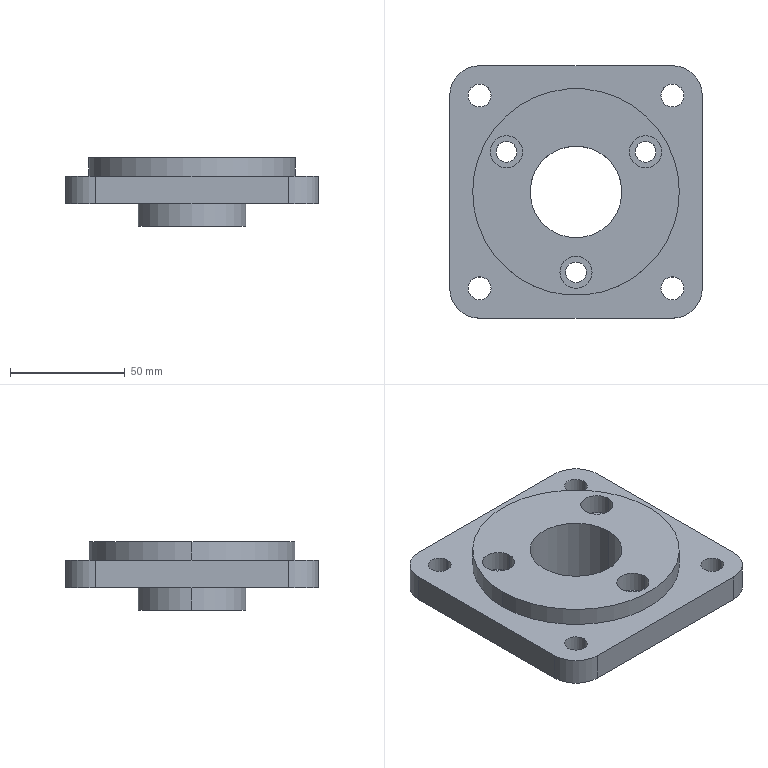Part | SolidWorks | features ICE 6, CirPattern 1, Extrusion 1 | 1 solid | 41 faces | box 110 x 110 x 29.8 mm | volume 163882 mm3 | cylinder 30 | plane 11 | commonest cylinder face diameters 10 x8 9 x6 14 x6 26 x4 40 x2 47 x2
STEP:
#1=CARTESIAN_POINT('',(-34.811,17.5,0.));
#2=VERTEX_POINT('',#1);
#3=CARTESIAN_POINT('',(-25.811,17.5,0.));
#4=VERTEX_POINT('',#3);
#5=CARTESIAN_POINT('',(-30.311,17.5,0.));
#6=DIRECTION('',(0.,0.,1.));
#7=DIRECTION('',(1.,0.,0.));
#8=AXIS2_PLACEMENT_3D('',#5,#6,#7);
#9=CIRCLE('',#8,4.5);
#10=EDGE_CURVE('',#2,#4,#9,.T.);
#11=ORIENTED_EDGE('',*,*,#10,.F.);
#12=CARTESIAN_POINT('',(-34.811,17.5,11.));
#13=VERTEX_POINT('',#12);
#14=CARTESIAN_POINT('',(-34.811,17.5,-790.));
#15=DIRECTION('',(0.,0.,1.));
#16=VECTOR('',#15,1000.);
#17=LINE('',#14,#16);
#18=EDGE_CURVE('',#2,#13,#17,.T.);
#19=ORIENTED_EDGE('',*,*,#18,.T.);
#20=CARTESIAN_POINT('',(-25.811,17.5,11.));
#21=VERTEX_POINT('',#20);
#22=CARTESIAN_POINT('',(-30.311,17.5,11.));
#23=DIRECTION('',(0.,0.,1.));
#24=DIRECTION('',(-0.5,-0.866,0.));
#25=AXIS2_PLACEMENT_3D('',#22,#23,#24);
#26=CIRCLE('',#25,4.5);
#27=EDGE_CURVE('',#13,#21,#26,.T.);
#28=ORIENTED_EDGE('',*,*,#27,.T.);
#29=CARTESIAN_POINT('',(-25.811,17.5,-790.));
#30=DIRECTION('',(0.,0.,1.));
#31=VECTOR('',#30,1000.);
#32=LINE('',#29,#31);
#33=EDGE_CURVE('',#4,#21,#32,.T.);
#34=ORIENTED_EDGE('',*,*,#33,.F.);
#35=EDGE_LOOP('',(#11,#19,#28,#34));
#36=FACE_OUTER_BOUND('',#35,.T.);
#37=CARTESIAN_POINT('',(-30.311,17.5,-790.));
#38=DIRECTION('',(0.,0.,1.));
#39=DIRECTION('',(1.,0.,0.));
#40=AXIS2_PLACEMENT_3D('',#37,#38,#39);
#41=CYLINDRICAL_SURFACE('',#40,4.5);
#42=ADVANCED_FACE('',(#36),#41,.F.);
#43=CARTESIAN_POINT('',(25.811,17.5,0.));
#44=VERTEX_POINT('',#43);
#45=CARTESIAN_POINT('',(34.811,17.5,0.));
#46=VERTEX_POINT('',#45);
#47=CARTESIAN_POINT('',(30.311,17.5,0.));
#48=DIRECTION('',(0.,0.,1.));
#49=DIRECTION('',(1.,0.,0.));
#50=AXIS2_PLACEMENT_3D('',#47,#48,#49);
#51=CIRCLE('',#50,4.5);
#52=EDGE_CURVE('',#44,#46,#51,.T.);
#53=ORIENTED_EDGE('',*,*,#52,.F.);
#54=CARTESIAN_POINT('',(25.811,17.5,11.));
#55=VERTEX_POINT('',#54);
#56=CARTESIAN_POINT('',(25.811,17.5,-790.));
#57=DIRECTION('',(0.,0.,1.));
#58=VECTOR('',#57,1000.);
#59=LINE('',#56,#58);
#60=EDGE_CURVE('',#44,#55,#59,.T.);
#61=ORIENTED_EDGE('',*,*,#60,.T.);
#62=CARTESIAN_POINT('',(34.811,17.5,11.));
#63=VERTEX_POINT('',#62);
#64=CARTESIAN_POINT('',(30.311,17.5,11.));
#65=DIRECTION('',(0.,0.,1.));
#66=DIRECTION('',(-0.5,0.866,0.));
#67=AXIS2_PLACEMENT_3D('',#64,#65,#66);
#68=CIRCLE('',#67,4.5);
#69=EDGE_CURVE('',#55,#63,#68,.T.);
#70=ORIENTED_EDGE('',*,*,#69,.T.);
#71=CARTESIAN_POINT('',(34.811,17.5,-790.));
#72=DIRECTION('',(0.,0.,1.));
#73=VECTOR('',#72,1000.);
#74=LINE('',#71,#73);
#75=EDGE_CURVE('',#46,#63,#74,.T.);
#76=ORIENTED_EDGE('',*,*,#75,.F.);
#77=EDGE_LOOP('',(#53,#61,#70,#76));
#78=FACE_OUTER_BOUND('',#77,.T.);
#79=CARTESIAN_POINT('',(30.311,17.5,-790.));
#80=DIRECTION('',(0.,0.,1.));
#81=DIRECTION('',(1.,0.,0.));
#82=AXIS2_PLACEMENT_3D('',#79,#80,#81);
#83=CYLINDRICAL_SURFACE('',#82,4.5);
#84=ADVANCED_FACE('',(#78),#83,.F.);
#85=CARTESIAN_POINT('',(-37.311,17.5,11.));
#86=VERTEX_POINT('',#85);
#87=CARTESIAN_POINT('',(-23.311,17.5,11.));
#88=VERTEX_POINT('',#87);
#89=CARTESIAN_POINT('',(-30.311,17.5,11.));
#90=DIRECTION('',(0.,0.,1.));
#91=DIRECTION('',(-0.5,-0.866,0.));
#92=AXIS2_PLACEMENT_3D('',#89,#90,#91);
#93=CIRCLE('',#92,7.);
#94=EDGE_CURVE('',#86,#88,#93,.T.);
#95=ORIENTED_EDGE('',*,*,#94,.F.);
#96=CARTESIAN_POINT('',(-37.311,17.5,20.));
#97=VERTEX_POINT('',#96);
#98=CARTESIAN_POINT('',(-37.311,17.5,11.));
#99=DIRECTION('',(0.,0.,1.));
#100=VECTOR('',#99,1000.);
#101=LINE('',#98,#100);
#102=EDGE_CURVE('',#86,#97,#101,.T.);
#103=ORIENTED_EDGE('',*,*,#102,.T.);
#104=CARTESIAN_POINT('',(-23.311,17.5,20.));
#105=VERTEX_POINT('',#104);
#106=CARTESIAN_POINT('',(-30.311,17.5,20.));
#107=DIRECTION('',(0.,0.,1.));
#108=DIRECTION('',(-0.5,-0.866,0.));
#109=AXIS2_PLACEMENT_3D('',#106,#107,#108);
#110=CIRCLE('',#109,7.);
#111=EDGE_CURVE('',#97,#105,#110,.T.);
#112=ORIENTED_EDGE('',*,*,#111,.T.);
#113=CARTESIAN_POINT('',(-23.311,17.5,11.));
#114=DIRECTION('',(0.,0.,1.));
#115=VECTOR('',#114,1000.);
#116=LINE('',#113,#115);
#117=EDGE_CURVE('',#88,#105,#116,.T.);
#118=ORIENTED_EDGE('',*,*,#117,.F.);
#119=EDGE_LOOP('',(#95,#103,#112,#118));
#120=FACE_OUTER_BOUND('',#119,.T.);
#121=CARTESIAN_POINT('',(-30.311,17.5,11.));
#122=DIRECTION('',(0.,0.,1.));
#123=DIRECTION('',(1.,0.,0.));
#124=AXIS2_PLACEMENT_3D('',#121,#122,#123);
#125=CYLINDRICAL_SURFACE('',#124,7.);
#126=ADVANCED_FACE('',(#120),#125,.F.);
#127=CARTESIAN_POINT('',(23.311,17.5,11.));
#128=VERTEX_POINT('',#127);
#129=CARTESIAN_POINT('',(37.311,17.5,11.));
#130=VERTEX_POINT('',#129);
#131=CARTESIAN_POINT('',(30.311,17.5,11.));
#132=DIRECTION('',(0.,0.,1.));
#133=DIRECTION('',(-0.5,0.866,0.));
#134=AXIS2_PLACEMENT_3D('',#131,#132,#133);
#135=CIRCLE('',#134,7.);
#136=EDGE_CURVE('',#128,#130,#135,.T.);
#137=ORIENTED_EDGE('',*,*,#136,.F.);
#138=CARTESIAN_POINT('',(23.311,17.5,20.));
#139=VERTEX_POINT('',#138);
#140=CARTESIAN_POINT('',(23.311,17.5,11.));
#141=DIRECTION('',(0.,0.,1.));
#142=VECTOR('',#141,1000.);
#143=LINE('',#140,#142);
#144=EDGE_CURVE('',#128,#139,#143,.T.);
#145=ORIENTED_EDGE('',*,*,#144,.T.);
#146=CARTESIAN_POINT('',(37.311,17.5,20.));
#147=VERTEX_POINT('',#146);
#148=CARTESIAN_POINT('',(30.311,17.5,20.));
#149=DIRECTION('',(0.,0.,1.));
#150=DIRECTION('',(-0.5,0.866,0.));
#151=AXIS2_PLACEMENT_3D('',#148,#149,#150);
#152=CIRCLE('',#151,7.);
#153=EDGE_CURVE('',#139,#147,#152,.T.);
#154=ORIENTED_EDGE('',*,*,#153,.T.);
#155=CARTESIAN_POINT('',(37.311,17.5,11.));
#156=DIRECTION('',(0.,0.,1.));
#157=VECTOR('',#156,1000.);
#158=LINE('',#155,#157);
#159=EDGE_CURVE('',#130,#147,#158,.T.);
#160=ORIENTED_EDGE('',*,*,#159,.F.);
#161=EDGE_LOOP('',(#137,#145,#154,#160));
#162=FACE_OUTER_BOUND('',#161,.T.);
#163=CARTESIAN_POINT('',(30.311,17.5,11.));
#164=DIRECTION('',(0.,0.,1.));
#165=DIRECTION('',(1.,0.,0.));
#166=AXIS2_PLACEMENT_3D('',#163,#164,#165);
#167=CYLINDRICAL_SURFACE('',#166,7.);
#168=ADVANCED_FACE('',(#162),#167,.F.);
#169=CARTESIAN_POINT('',(-4.5,-35.,0.));
#170=VERTEX_POINT('',#169);
#171=CARTESIAN_POINT('',(4.5,-35.,0.));
#172=VERTEX_POINT('',#171);
#173=CARTESIAN_POINT('',(0.,-35.,0.));
#174=DIRECTION('',(0.,0.,1.));
#175=DIRECTION('',(1.,0.,0.));
#176=AXIS2_PLACEMENT_3D('',#173,#174,#175);
#177=CIRCLE('',#176,4.5);
#178=EDGE_CURVE('',#170,#172,#177,.T.);
#179=ORIENTED_EDGE('',*,*,#178,.F.);
#180=CARTESIAN_POINT('',(-4.5,-35.,11.));
#181=VERTEX_POINT('',#180);
#182=CARTESIAN_POINT('',(-4.5,-35.,-790.));
#183=DIRECTION('',(0.,0.,1.));
#184=VECTOR('',#183,1000.);
#185=LINE('',#182,#184);
#186=EDGE_CURVE('',#170,#181,#185,.T.);
#187=ORIENTED_EDGE('',*,*,#186,.T.);
#188=CARTESIAN_POINT('',(4.5,-35.,11.));
#189=VERTEX_POINT('',#188);
#190=CARTESIAN_POINT('',(0.,-35.,11.));
#191=DIRECTION('',(0.,0.,1.));
#192=DIRECTION('',(1.,0.,0.));
#193=AXIS2_PLACEMENT_3D('',#190,#191,#192);
#194=CIRCLE('',#193,4.5);
#195=EDGE_CURVE('',#181,#189,#194,.T.);
#196=ORIENTED_EDGE('',*,*,#195,.T.);
#197=CARTESIAN_POINT('',(4.5,-35.,-790.));
#198=DIRECTION('',(0.,0.,1.));
#199=VECTOR('',#198,1000.);
#200=LINE('',#197,#199);
#201=EDGE_CURVE('',#172,#189,#200,.T.);
#202=ORIENTED_EDGE('',*,*,#201,.F.);
#203=EDGE_LOOP('',(#179,#187,#196,#202));
#204=FACE_OUTER_BOUND('',#203,.T.);
#205=CARTESIAN_POINT('',(0.,-35.,-790.));
#206=DIRECTION('',(0.,0.,1.));
#207=DIRECTION('',(1.,0.,0.));
#208=AXIS2_PLACEMENT_3D('',#205,#206,#207);
#209=CYLINDRICAL_SURFACE('',#208,4.5);
#210=ADVANCED_FACE('',(#204),#209,.F.);
#211=CARTESIAN_POINT('',(-7.,-35.,11.));
#212=VERTEX_POINT('',#211);
#213=CARTESIAN_POINT('',(7.,-35.,11.));
#214=VERTEX_POINT('',#213);
#215=CARTESIAN_POINT('',(0.,-35.,11.));
#216=DIRECTION('',(0.,0.,1.));
#217=DIRECTION('',(1.,0.,0.));
#218=AXIS2_PLACEMENT_3D('',#215,#216,#217);
#219=CIRCLE('',#218,7.);
#220=EDGE_CURVE('',#212,#214,#219,.T.);
#221=ORIENTED_EDGE('',*,*,#220,.F.);
#222=CARTESIAN_POINT('',(-7.,-35.,20.));
#223=VERTEX_POINT('',#222);
#224=CARTESIAN_POINT('',(-7.,-35.,11.));
#225=DIRECTION('',(0.,0.,1.));
#226=VECTOR('',#225,1000.);
#227=LINE('',#224,#226);
#228=EDGE_CURVE('',#212,#223,#227,.T.);
#229=ORIENTED_EDGE('',*,*,#228,.T.);
#230=CARTESIAN_POINT('',(7.,-35.,20.));
#231=VERTEX_POINT('',#230);
#232=CARTESIAN_POINT('',(0.,-35.,20.));
#233=DIRECTION('',(0.,0.,1.));
#234=DIRECTION('',(1.,0.,0.));
#235=AXIS2_PLACEMENT_3D('',#232,#233,#234);
#236=CIRCLE('',#235,7.);
#237=EDGE_CURVE('',#223,#231,#236,.T.);
#238=ORIENTED_EDGE('',*,*,#237,.T.);
#239=CARTESIAN_POINT('',(7.,-35.,11.));
#240=DIRECTION('',(0.,0.,1.));
#241=VECTOR('',#240,1000.);
#242=LINE('',#239,#241);
#243=EDGE_CURVE('',#214,#231,#242,.T.);
#244=ORIENTED_EDGE('',*,*,#243,.F.);
#245=EDGE_LOOP('',(#221,#229,#238,#244));
#246=FACE_OUTER_BOUND('',#245,.T.);
#247=CARTESIAN_POINT('',(0.,-35.,11.));
#248=DIRECTION('',(0.,0.,1.));
#249=DIRECTION('',(1.,0.,0.));
#250=AXIS2_PLACEMENT_3D('',#247,#248,#249);
#251=CYLINDRICAL_SURFACE('',#250,7.);
#252=ADVANCED_FACE('',(#246),#251,.F.);
#253=CARTESIAN_POINT('',(-20.,0.,20.));
#254=VERTEX_POINT('',#253);
#255=CARTESIAN_POINT('',(20.,0.,20.));
#256=VERTEX_POINT('',#255);
#257=CARTESIAN_POINT('',(0.,0.,20.));
#258=DIRECTION('',(0.,0.,1.));
#259=DIRECTION('',(1.,0.,0.));
#260=AXIS2_PLACEMENT_3D('',#257,#258,#259);
#261=CIRCLE('',#260,20.);
#262=EDGE_CURVE('',#254,#256,#261,.T.);
#263=ORIENTED_EDGE('',*,*,#262,.T.);
#264=CARTESIAN_POINT('',(20.,0.,-9.8));
#265=VERTEX_POINT('',#264);
#266=CARTESIAN_POINT('',(20.,0.,70.2));
#267=DIRECTION('',(0.,0.,-1.));
#268=VECTOR('',#267,1000.);
#269=LINE('',#266,#268);
#270=EDGE_CURVE('',#256,#265,#269,.T.);
#271=ORIENTED_EDGE('',*,*,#270,.T.);
#272=CARTESIAN_POINT('',(-20.,0.,-9.8));
#273=VERTEX_POINT('',#272);
#274=CARTESIAN_POINT('',(0.,0.,-9.8));
#275=DIRECTION('',(0.,0.,-1.));
#276=DIRECTION('',(-1.,0.,0.));
#277=AXIS2_PLACEMENT_3D('',#274,#275,#276);
#278=CIRCLE('',#277,20.);
#279=EDGE_CURVE('',#265,#273,#278,.T.);
#280=ORIENTED_EDGE('',*,*,#279,.T.);
#281=CARTESIAN_POINT('',(-20.,0.,70.2));
#282=DIRECTION('',(0.,0.,-1.));
#283=VECTOR('',#282,1000.);
#284=LINE('',#281,#283);
#285=EDGE_CURVE('',#254,#273,#284,.T.);
#286=ORIENTED_EDGE('',*,*,#285,.F.);
#287=EDGE_LOOP('',(#263,#271,#280,#286));
#288=FACE_OUTER_BOUND('',#287,.T.);
#289=CARTESIAN_POINT('',(0.,0.,70.2));
#290=DIRECTION('',(0.,0.,-1.));
#291=DIRECTION('',(-1.,0.,0.));
#292=AXIS2_PLACEMENT_3D('',#289,#290,#291);
#293=CYLINDRICAL_SURFACE('',#292,20.);
#294=ADVANCED_FACE('',(#288),#293,.F.);
#295=CARTESIAN_POINT('',(-23.5,0.,-9.8));
#296=VERTEX_POINT('',#295);
#297=CARTESIAN_POINT('',(23.5,0.,-9.8));
#298=VERTEX_POINT('',#297);
#299=CARTESIAN_POINT('',(0.,0.,-9.8));
#300=DIRECTION('',(0.,0.,-1.));
#301=DIRECTION('',(-1.,0.,0.));
#302=AXIS2_PLACEMENT_3D('',#299,#300,#301);
#303=CIRCLE('',#302,23.5);
#304=EDGE_CURVE('',#296,#298,#303,.T.);
#305=ORIENTED_EDGE('',*,*,#304,.F.);
#306=CARTESIAN_POINT('',(-23.5,0.,0.));
#307=VERTEX_POINT('',#306);
#308=CARTESIAN_POINT('',(-23.5,0.,-9.8));
#309=DIRECTION('',(0.,0.,1.));
#310=VECTOR('',#309,1000.);
#311=LINE('',#308,#310);
#312=EDGE_CURVE('',#296,#307,#311,.T.);
#313=ORIENTED_EDGE('',*,*,#312,.T.);
#314=CARTESIAN_POINT('',(23.5,0.,0.));
#315=VERTEX_POINT('',#314);
#316=CARTESIAN_POINT('',(0.,0.,0.));
#317=DIRECTION('',(0.,0.,-1.));
#318=DIRECTION('',(1.,0.,0.));
#319=AXIS2_PLACEMENT_3D('',#316,#317,#318);
#320=CIRCLE('',#319,23.5);
#321=EDGE_CURVE('',#307,#315,#320,.T.);
#322=ORIENTED_EDGE('',*,*,#321,.T.);
#323=CARTESIAN_POINT('',(23.5,0.,-9.8));
#324=DIRECTION('',(0.,0.,1.));
#325=VECTOR('',#324,1000.);
#326=LINE('',#323,#325);
#327=EDGE_CURVE('',#298,#315,#326,.T.);
#328=ORIENTED_EDGE('',*,*,#327,.F.);
#329=EDGE_LOOP('',(#305,#313,#322,#328));
#330=FACE_OUTER_BOUND('',#329,.T.);
#331=CARTESIAN_POINT('',(0.,0.,-9.8));
#332=DIRECTION('',(0.,0.,1.));
#333=DIRECTION('',(1.,0.,0.));
#334=AXIS2_PLACEMENT_3D('',#331,#332,#333);
#335=CYLINDRICAL_SURFACE('',#334,23.5);
#336=ADVANCED_FACE('',(#330),#335,.T.);
#337=CARTESIAN_POINT('',(45.,0.,20.));
#338=VERTEX_POINT('',#337);
#339=CARTESIAN_POINT('',(-45.,0.,20.));
#340=VERTEX_POINT('',#339);
#341=CARTESIAN_POINT('',(0.,0.,20.));
#342=DIRECTION('',(0.,0.,1.));
#343=DIRECTION('',(1.,0.,0.));
#344=AXIS2_PLACEMENT_3D('',#341,#342,#343);
#345=CIRCLE('',#344,45.);
#346=EDGE_CURVE('',#338,#340,#345,.T.);
#347=ORIENTED_EDGE('',*,*,#346,.F.);
#348=CARTESIAN_POINT('',(45.,0.,12.));
#349=VERTEX_POINT('',#348);
#350=CARTESIAN_POINT('',(45.,0.,20.));
#351=DIRECTION('',(0.,0.,-1.));
#352=VECTOR('',#351,1000.);
#353=LINE('',#350,#352);
#354=EDGE_CURVE('',#338,#349,#353,.T.);
#355=ORIENTED_EDGE('',*,*,#354,.T.);
#356=CARTESIAN_POINT('',(-45.,0.,12.));
#357=VERTEX_POINT('',#356);
#358=CARTESIAN_POINT('',(0.,0.,12.));
#359=DIRECTION('',(0.,0.,1.));
#360=DIRECTION('',(1.,0.,0.));
#361=AXIS2_PLACEMENT_3D('',#358,#359,#360);
#362=CIRCLE('',#361,45.);
#363=EDGE_CURVE('',#349,#357,#362,.T.);
#364=ORIENTED_EDGE('',*,*,#363,.T.);
#365=CARTESIAN_POINT('',(-45.,0.,20.));
#366=DIRECTION('',(0.,0.,-1.));
#367=VECTOR('',#366,1000.);
#368=LINE('',#365,#367);
#369=EDGE_CURVE('',#340,#357,#368,.T.);
#370=ORIENTED_EDGE('',*,*,#369,.F.);
#371=EDGE_LOOP('',(#347,#355,#364,#370));
#372=FACE_OUTER_BOUND('',#371,.T.);
#373=CARTESIAN_POINT('',(0.,0.,20.));
#374=DIRECTION('',(0.,0.,-1.));
#375=DIRECTION('',(-1.,0.,0.));
#376=AXIS2_PLACEMENT_3D('',#373,#374,#375);
#377=CYLINDRICAL_SURFACE('',#376,45.);
#378=ADVANCED_FACE('',(#372),#377,.T.);
#379=CARTESIAN_POINT('',(-47.,42.,0.));
#380=VERTEX_POINT('',#379);
#381=CARTESIAN_POINT('',(-37.,42.,0.));
#382=VERTEX_POINT('',#381);
#383=CARTESIAN_POINT('',(-42.,42.,0.));
#384=DIRECTION('',(0.,0.,1.));
#385=DIRECTION('',(1.,0.,0.));
#386=AXIS2_PLACEMENT_3D('',#383,#384,#385);
#387=CIRCLE('',#386,5.);
#388=EDGE_CURVE('',#380,#382,#387,.T.);
#389=ORIENTED_EDGE('',*,*,#388,.F.);
#390=CARTESIAN_POINT('',(-47.,42.,12.));
#391=VERTEX_POINT('',#390);
#392=CARTESIAN_POINT('',(-47.,42.,-38.));
#393=DIRECTION('',(0.,0.,1.));
#394=VECTOR('',#393,1000.);
#395=LINE('',#392,#394);
#396=EDGE_CURVE('',#380,#391,#395,.T.);
#397=ORIENTED_EDGE('',*,*,#396,.T.);
#398=CARTESIAN_POINT('',(-37.,42.,12.));
#399=VERTEX_POINT('',#398);
#400=CARTESIAN_POINT('',(-42.,42.,12.));
#401=DIRECTION('',(0.,0.,1.));
#402=DIRECTION('',(1.,0.,0.));
#403=AXIS2_PLACEMENT_3D('',#400,#401,#402);
#404=CIRCLE('',#403,5.);
#405=EDGE_CURVE('',#391,#399,#404,.T.);
#406=ORIENTED_EDGE('',*,*,#405,.T.);
#407=CARTESIAN_POINT('',(-37.,42.,-38.));
#408=DIRECTION('',(0.,0.,1.));
#409=VECTOR('',#408,1000.);
#410=LINE('',#407,#409);
#411=EDGE_CURVE('',#382,#399,#410,.T.);
#412=ORIENTED_EDGE('',*,*,#411,.F.);
#413=EDGE_LOOP('',(#389,#397,#406,#412));
#414=FACE_OUTER_BOUND('',#413,.T.);
#415=CARTESIAN_POINT('',(-42.,42.,-38.));
#416=DIRECTION('',(0.,0.,1.));
#417=DIRECTION('',(1.,0.,0.));
#418=AXIS2_PLACEMENT_3D('',#415,#416,#417);
#419=CYLINDRICAL_SURFACE('',#418,5.);
#420=ADVANCED_FACE('',(#414),#419,.F.);
#421=CARTESIAN_POINT('',(-47.,-42.,0.));
#422=VERTEX_POINT('',#421);
#423=CARTESIAN_POINT('',(-37.,-42.,0.));
#424=VERTEX_POINT('',#423);
#425=CARTESIAN_POINT('',(-42.,-42.,0.));
#426=DIRECTION('',(0.,0.,1.));
#427=DIRECTION('',(1.,0.,0.));
#428=AXIS2_PLACEMENT_3D('',#425,#426,#427);
#429=CIRCLE('',#428,5.);
#430=EDGE_CURVE('',#422,#424,#429,.T.);
#431=ORIENTED_EDGE('',*,*,#430,.F.);
#432=CARTESIAN_POINT('',(-47.,-42.,12.));
#433=VERTEX_POINT('',#432);
#434=CARTESIAN_POINT('',(-47.,-42.,-38.));
#435=DIRECTION('',(0.,0.,1.));
#436=VECTOR('',#435,1000.);
#437=LINE('',#434,#436);
#438=EDGE_CURVE('',#422,#433,#437,.T.);
#439=ORIENTED_EDGE('',*,*,#438,.T.);
#440=CARTESIAN_POINT('',(-37.,-42.,12.));
#441=VERTEX_POINT('',#440);
#442=CARTESIAN_POINT('',(-42.,-42.,12.));
#443=DIRECTION('',(0.,0.,1.));
#444=DIRECTION('',(1.,0.,0.));
#445=AXIS2_PLACEMENT_3D('',#442,#443,#444);
#446=CIRCLE('',#445,5.);
#447=EDGE_CURVE('',#433,#441,#446,.T.);
#448=ORIENTED_EDGE('',*,*,#447,.T.);
#449=CARTESIAN_POINT('',(-37.,-42.,-38.));
#450=DIRECTION('',(0.,0.,1.));
#451=VECTOR('',#450,1000.);
#452=LINE('',#449,#451);
#453=EDGE_CURVE('',#424,#441,#452,.T.);
#454=ORIENTED_EDGE('',*,*,#453,.F.);
#455=EDGE_LOOP('',(#431,#439,#448,#454));
#456=FACE_OUTER_BOUND('',#455,.T.);
#457=CARTESIAN_POINT('',(-42.,-42.,-38.));
#458=DIRECTION('',(0.,0.,1.));
#459=DIRECTION('',(1.,0.,0.));
#460=AXIS2_PLACEMENT_3D('',#457,#458,#459);
#461=CYLINDRICAL_SURFACE('',#460,5.);
#462=ADVANCED_FACE('',(#456),#461,.F.);
#463=CARTESIAN_POINT('',(37.,-42.,0.));
#464=VERTEX_POINT('',#463);
#465=CARTESIAN_POINT('',(47.,-42.,0.));
#466=VERTEX_POINT('',#465);
#467=CARTESIAN_POINT('',(42.,-42.,0.));
#468=DIRECTION('',(0.,0.,1.));
#469=DIRECTION('',(1.,0.,0.));
#470=AXIS2_PLACEMENT_3D('',#467,#468,#469);
#471=CIRCLE('',#470,5.);
#472=EDGE_CURVE('',#464,#466,#471,.T.);
#473=ORIENTED_EDGE('',*,*,#472,.F.);
#474=CARTESIAN_POINT('',(37.,-42.,12.));
#475=VERTEX_POINT('',#474);
#476=CARTESIAN_POINT('',(37.,-42.,-38.));
#477=DIRECTION('',(0.,0.,1.));
#478=VECTOR('',#477,1000.);
#479=LINE('',#476,#478);
#480=EDGE_CURVE('',#464,#475,#479,.T.);
#481=ORIENTED_EDGE('',*,*,#480,.T.);
#482=CARTESIAN_POINT('',(47.,-42.,12.));
#483=VERTEX_POINT('',#482);
#484=CARTESIAN_POINT('',(42.,-42.,12.));
#485=DIRECTION('',(0.,0.,1.));
#486=DIRECTION('',(1.,0.,0.));
#487=AXIS2_PLACEMENT_3D('',#484,#485,#486);
#488=CIRCLE('',#487,5.);
#489=EDGE_CURVE('',#475,#483,#488,.T.);
#490=ORIENTED_EDGE('',*,*,#489,.T.);
#491=CARTESIAN_POINT('',(47.,-42.,-38.));
#492=DIRECTION('',(0.,0.,1.));
#493=VECTOR('',#492,1000.);
#494=LINE('',#491,#493);
#495=EDGE_CURVE('',#466,#483,#494,.T.);
#496=ORIENTED_EDGE('',*,*,#495,.F.);
#497=EDGE_LOOP('',(#473,#481,#490,#496));
#498=FACE_OUTER_BOUND('',#497,.T.);
#499=CARTESIAN_POINT('',(42.,-42.,-38.));
#500=DIRECTION('',(0.,0.,1.));
#501=DIRECTION('',(1.,0.,0.));
#502=AXIS2_PLACEMENT_3D('',#499,#500,#501);
#503=CYLINDRICAL_SURFACE('',#502,5.);
#504=ADVANCED_FACE('',(#498),#503,.F.);
#505=CARTESIAN_POINT('',(37.,42.,0.));
#506=VERTEX_POINT('',#505);
#507=CARTESIAN_POINT('',(47.,42.,0.));
#508=VERTEX_POINT('',#507);
#509=CARTESIAN_POINT('',(42.,42.,0.));
#510=DIRECTION('',(0.,0.,1.));
#511=DIRECTION('',(1.,0.,0.));
#512=AXIS2_PLACEMENT_3D('',#509,#510,#511);
#513=CIRCLE('',#512,5.);
#514=EDGE_CURVE('',#506,#508,#513,.T.);
#515=ORIENTED_EDGE('',*,*,#514,.F.);
#516=CARTESIAN_POINT('',(37.,42.,12.));
#517=VERTEX_POINT('',#516);
#518=CARTESIAN_POINT('',(37.,42.,-38.));
#519=DIRECTION('',(0.,0.,1.));
#520=VECTOR('',#519,1000.);
#521=LINE('',#518,#520);
#522=EDGE_CURVE('',#506,#517,#521,.T.);
#523=ORIENTED_EDGE('',*,*,#522,.T.);
#524=CARTESIAN_POINT('',(47.,42.,12.));
#525=VERTEX_POINT('',#524);
#526=CARTESIAN_POINT('',(42.,42.,12.));
#527=DIRECTION('',(0.,0.,1.));
#528=DIRECTION('',(1.,0.,0.));
#529=AXIS2_PLACEMENT_3D('',#526,#527,#528);
#530=CIRCLE('',#529,5.);
#531=EDGE_CURVE('',#517,#525,#530,.T.);
#532=ORIENTED_EDGE('',*,*,#531,.T.);
#533=CARTESIAN_POINT('',(47.,42.,-38.));
#534=DIRECTION('',(0.,0.,1.));
#535=VECTOR('',#534,1000.);
#536=LINE('',#533,#535);
#537=EDGE_CURVE('',#508,#525,#536,.T.);
#538=ORIENTED_EDGE('',*,*,#537,.F.);
#539=EDGE_LOOP('',(#515,#523,#532,#538));
#540=FACE_OUTER_BOUND('',#539,.T.);
#541=CARTESIAN_POINT('',(42.,42.,-38.));
#542=DIRECTION('',(0.,0.,1.));
#543=DIRECTION('',(1.,0.,0.));
#544=AXIS2_PLACEMENT_3D('',#541,#542,#543);
#545=CYLINDRICAL_SURFACE('',#544,5.);
#546=ADVANCED_FACE('',(#540),#545,.F.);
#547=CARTESIAN_POINT('',(42.,-55.,0.));
#548=VERTEX_POINT('',#547);
#549=CARTESIAN_POINT('',(55.,-42.,0.));
#550=VERTEX_POINT('',#549);
#551=CARTESIAN_POINT('',(42.,-42.,0.));
#552=DIRECTION('',(0.,0.,1.));
#553=DIRECTION('',(1.,0.,0.));
#554=AXIS2_PLACEMENT_3D('',#551,#552,#553);
#555=CIRCLE('',#554,13.);
#556=EDGE_CURVE('',#548,#550,#555,.T.);
#557=ORIENTED_EDGE('',*,*,#556,.T.);
#558=CARTESIAN_POINT('',(55.,-42.,12.));
#559=VERTEX_POINT('',#558);
#560=CARTESIAN_POINT('',(55.,-42.,12.));
#561=DIRECTION('',(0.,0.,-1.));
#562=VECTOR('',#561,1000.);
#563=LINE('',#560,#562);
#564=EDGE_CURVE('',#559,#550,#563,.T.);
#565=ORIENTED_EDGE('',*,*,#564,.F.);
#566=CARTESIAN_POINT('',(42.,-55.,12.));
#567=VERTEX_POINT('',#566);
#568=CARTESIAN_POINT('',(42.,-42.,12.));
#569=DIRECTION('',(0.,0.,1.));
#570=DIRECTION('',(1.,0.,0.));
#571=AXIS2_PLACEMENT_3D('',#568,#569,#570);
#572=CIRCLE('',#571,13.);
#573=EDGE_CURVE('',#567,#559,#572,.T.);
#574=ORIENTED_EDGE('',*,*,#573,.F.);
#575=CARTESIAN_POINT('',(42.,-55.,12.));
#576=DIRECTION('',(0.,0.,-1.));
#577=VECTOR('',#576,1000.);
#578=LINE('',#575,#577);
#579=EDGE_CURVE('',#567,#548,#578,.T.);
#580=ORIENTED_EDGE('',*,*,#579,.T.);
#581=EDGE_LOOP('',(#557,#565,#574,#580));
#582=FACE_OUTER_BOUND('',#581,.T.);
#583=CARTESIAN_POINT('',(42.,-42.,12.));
#584=DIRECTION('',(0.,0.,-1.));
#585=DIRECTION('',(-1.,0.,0.));
#586=AXIS2_PLACEMENT_3D('',#583,#584,#585);
#587=CYLINDRICAL_SURFACE('',#586,13.);
#588=ADVANCED_FACE('',(#582),#587,.T.);
#589=CARTESIAN_POINT('',(55.,42.,0.));
#590=VERTEX_POINT('',#589);
#591=CARTESIAN_POINT('',(55.,-42.,0.));
#592=DIRECTION('',(0.,1.,0.));
#593=VECTOR('',#592,1000.);
#594=LINE('',#591,#593);
#595=EDGE_CURVE('',#550,#590,#594,.T.);
#596=ORIENTED_EDGE('',*,*,#595,.T.);
#597=CARTESIAN_POINT('',(55.,42.,12.));
#598=VERTEX_POINT('',#597);
#599=CARTESIAN_POINT('',(55.,42.,12.));
#600=DIRECTION('',(0.,0.,-1.));
#601=VECTOR('',#600,1000.);
#602=LINE('',#599,#601);
#603=EDGE_CURVE('',#598,#590,#602,.T.);
#604=ORIENTED_EDGE('',*,*,#603,.F.);
#605=CARTESIAN_POINT('',(55.,-42.,12.));
#606=DIRECTION('',(0.,1.,0.));
#607=VECTOR('',#606,1000.);
#608=LINE('',#605,#607);
#609=EDGE_CURVE('',#559,#598,#608,.T.);
#610=ORIENTED_EDGE('',*,*,#609,.F.);
#611=ORIENTED_EDGE('',*,*,#564,.T.);
#612=EDGE_LOOP('',(#596,#604,#610,#611));
#613=FACE_OUTER_BOUND('',#612,.T.);
#614=CARTESIAN_POINT('',(55.,-42.,12.));
#615=DIRECTION('',(-1.,0.,0.));
#616=DIRECTION('',(0.,0.,1.));
#617=AXIS2_PLACEMENT_3D('',#614,#615,#616);
#618=PLANE('',#617);
#619=ADVANCED_FACE('',(#613),#618,.F.);
#620=CARTESIAN_POINT('',(42.,55.,0.));
#621=VERTEX_POINT('',#620);
#622=CARTESIAN_POINT('',(42.,42.,0.));
#623=DIRECTION('',(0.,0.,1.));
#624=DIRECTION('',(-1.,0.,0.));
#625=AXIS2_PLACEMENT_3D('',#622,#623,#624);
#626=CIRCLE('',#625,13.);
#627=EDGE_CURVE('',#590,#621,#626,.T.);
#628=ORIENTED_EDGE('',*,*,#627,.T.);
#629=CARTESIAN_POINT('',(42.,55.,12.));
#630=VERTEX_POINT('',#629);
#631=CARTESIAN_POINT('',(42.,55.,12.));
#632=DIRECTION('',(0.,0.,-1.));
#633=VECTOR('',#632,1000.);
#634=LINE('',#631,#633);
#635=EDGE_CURVE('',#630,#621,#634,.T.);
#636=ORIENTED_EDGE('',*,*,#635,.F.);
#637=CARTESIAN_POINT('',(42.,42.,12.));
#638=DIRECTION('',(0.,0.,1.));
#639=DIRECTION('',(-1.,0.,0.));
#640=AXIS2_PLACEMENT_3D('',#637,#638,#639);
#641=CIRCLE('',#640,13.);
#642=EDGE_CURVE('',#598,#630,#641,.T.);
#643=ORIENTED_EDGE('',*,*,#642,.F.);
#644=ORIENTED_EDGE('',*,*,#603,.T.);
#645=EDGE_LOOP('',(#628,#636,#643,#644));
#646=FACE_OUTER_BOUND('',#645,.T.);
#647=CARTESIAN_POINT('',(42.,42.,12.));
#648=DIRECTION('',(0.,0.,-1.));
#649=DIRECTION('',(-1.,0.,0.));
#650=AXIS2_PLACEMENT_3D('',#647,#648,#649);
#651=CYLINDRICAL_SURFACE('',#650,13.);
#652=ADVANCED_FACE('',(#646),#651,.T.);
#653=CARTESIAN_POINT('',(-42.,55.,0.));
#654=VERTEX_POINT('',#653);
#655=CARTESIAN_POINT('',(-42.,55.,0.));
#656=DIRECTION('',(-1.,0.,0.));
#657=VECTOR('',#656,1000.);
#658=LINE('',#655,#657);
#659=EDGE_CURVE('',#621,#654,#658,.T.);
#660=ORIENTED_EDGE('',*,*,#659,.T.);
#661=CARTESIAN_POINT('',(-42.,55.,12.));
#662=VERTEX_POINT('',#661);
#663=CARTESIAN_POINT('',(-42.,55.,12.));
#664=DIRECTION('',(0.,0.,-1.));
#665=VECTOR('',#664,1000.);
#666=LINE('',#663,#665);
#667=EDGE_CURVE('',#662,#654,#666,.T.);
#668=ORIENTED_EDGE('',*,*,#667,.F.);
#669=CARTESIAN_POINT('',(-42.,55.,12.));
#670=DIRECTION('',(-1.,0.,0.));
#671=VECTOR('',#670,1000.);
#672=LINE('',#669,#671);
#673=EDGE_CURVE('',#630,#662,#672,.T.);
#674=ORIENTED_EDGE('',*,*,#673,.F.);
#675=ORIENTED_EDGE('',*,*,#635,.T.);
#676=EDGE_LOOP('',(#660,#668,#674,#675));
#677=FACE_OUTER_BOUND('',#676,.T.);
#678=CARTESIAN_POINT('',(-42.,55.,12.));
#679=DIRECTION('',(0.,-1.,0.));
#680=DIRECTION('',(0.,0.,-1.));
#681=AXIS2_PLACEMENT_3D('',#678,#679,#680);
#682=PLANE('',#681);
#683=ADVANCED_FACE('',(#677),#682,.F.);
#684=CARTESIAN_POINT('',(-55.,42.,0.));
#685=VERTEX_POINT('',#684);
#686=CARTESIAN_POINT('',(-42.,42.,0.));
#687=DIRECTION('',(0.,0.,1.));
#688=DIRECTION('',(-1.,0.,0.));
#689=AXIS2_PLACEMENT_3D('',#686,#687,#688);
#690=CIRCLE('',#689,13.);
#691=EDGE_CURVE('',#654,#685,#690,.T.);
#692=ORIENTED_EDGE('',*,*,#691,.T.);
#693=CARTESIAN_POINT('',(-55.,42.,12.));
#694=VERTEX_POINT('',#693);
#695=CARTESIAN_POINT('',(-55.,42.,12.));
#696=DIRECTION('',(0.,0.,-1.));
#697=VECTOR('',#696,1000.);
#698=LINE('',#695,#697);
#699=EDGE_CURVE('',#694,#685,#698,.T.);
#700=ORIENTED_EDGE('',*,*,#699,.F.);
#701=CARTESIAN_POINT('',(-42.,42.,12.));
#702=DIRECTION('',(0.,0.,1.));
#703=DIRECTION('',(-1.,0.,0.));
#704=AXIS2_PLACEMENT_3D('',#701,#702,#703);
#705=CIRCLE('',#704,13.);
#706=EDGE_CURVE('',#662,#694,#705,.T.);
#707=ORIENTED_EDGE('',*,*,#706,.F.);
#708=ORIENTED_EDGE('',*,*,#667,.T.);
#709=EDGE_LOOP('',(#692,#700,#707,#708));
#710=FACE_OUTER_BOUND('',#709,.T.);
#711=CARTESIAN_POINT('',(-42.,42.,12.));
#712=DIRECTION('',(0.,0.,-1.));
#713=DIRECTION('',(-1.,0.,0.));
#714=AXIS2_PLACEMENT_3D('',#711,#712,#713);
#715=CYLINDRICAL_SURFACE('',#714,13.);
#716=ADVANCED_FACE('',(#710),#715,.T.);
#717=CARTESIAN_POINT('',(-55.,-42.,0.));
#718=VERTEX_POINT('',#717);
#719=CARTESIAN_POINT('',(-55.,-42.,0.));
#720=DIRECTION('',(0.,-1.,0.));
#721=VECTOR('',#720,1000.);
#722=LINE('',#719,#721);
#723=EDGE_CURVE('',#685,#718,#722,.T.);
#724=ORIENTED_EDGE('',*,*,#723,.T.);
#725=CARTESIAN_POINT('',(-55.,-42.,12.));
#726=VERTEX_POINT('',#725);
#727=CARTESIAN_POINT('',(-55.,-42.,12.));
#728=DIRECTION('',(0.,0.,-1.));
#729=VECTOR('',#728,1000.);
#730=LINE('',#727,#729);
#731=EDGE_CURVE('',#726,#718,#730,.T.);
#732=ORIENTED_EDGE('',*,*,#731,.F.);
#733=CARTESIAN_POINT('',(-55.,-42.,12.));
#734=DIRECTION('',(0.,-1.,0.));
#735=VECTOR('',#734,1000.);
#736=LINE('',#733,#735);
#737=EDGE_CURVE('',#694,#726,#736,.T.);
#738=ORIENTED_EDGE('',*,*,#737,.F.);
#739=ORIENTED_EDGE('',*,*,#699,.T.);
#740=EDGE_LOOP('',(#724,#732,#738,#739));
#741=FACE_OUTER_BOUND('',#740,.T.);
#742=CARTESIAN_POINT('',(-55.,-42.,12.));
#743=DIRECTION('',(1.,0.,0.));
#744=DIRECTION('',(0.,0.,-1.));
#745=AXIS2_PLACEMENT_3D('',#742,#743,#744);
#746=PLANE('',#745);
#747=ADVANCED_FACE('',(#741),#746,.F.);
#748=CARTESIAN_POINT('',(-42.,-55.,0.));
#749=VERTEX_POINT('',#748);
#750=CARTESIAN_POINT('',(-42.,-42.,0.));
#751=DIRECTION('',(0.,0.,1.));
#752=DIRECTION('',(-1.,0.,0.));
#753=AXIS2_PLACEMENT_3D('',#750,#751,#752);
#754=CIRCLE('',#753,13.);
#755=EDGE_CURVE('',#718,#749,#754,.T.);
#756=ORIENTED_EDGE('',*,*,#755,.T.);
#757=CARTESIAN_POINT('',(-42.,-55.,12.));
#758=VERTEX_POINT('',#757);
#759=CARTESIAN_POINT('',(-42.,-55.,12.));
#760=DIRECTION('',(0.,0.,-1.));
#761=VECTOR('',#760,1000.);
#762=LINE('',#759,#761);
#763=EDGE_CURVE('',#758,#749,#762,.T.);
#764=ORIENTED_EDGE('',*,*,#763,.F.);
#765=CARTESIAN_POINT('',(-42.,-42.,12.));
#766=DIRECTION('',(0.,0.,1.));
#767=DIRECTION('',(-1.,0.,0.));
#768=AXIS2_PLACEMENT_3D('',#765,#766,#767);
#769=CIRCLE('',#768,13.);
#770=EDGE_CURVE('',#726,#758,#769,.T.);
#771=ORIENTED_EDGE('',*,*,#770,.F.);
#772=ORIENTED_EDGE('',*,*,#731,.T.);
#773=EDGE_LOOP('',(#756,#764,#771,#772));
#774=FACE_OUTER_BOUND('',#773,.T.);
#775=CARTESIAN_POINT('',(-42.,-42.,12.));
#776=DIRECTION('',(0.,0.,-1.));
#777=DIRECTION('',(-1.,0.,0.));
#778=AXIS2_PLACEMENT_3D('',#775,#776,#777);
#779=CYLINDRICAL_SURFACE('',#778,13.);
#780=ADVANCED_FACE('',(#774),#779,.T.);
#781=CARTESIAN_POINT('',(-42.,-55.,0.));
#782=DIRECTION('',(1.,0.,0.));
#783=VECTOR('',#782,1000.);
#784=LINE('',#781,#783);
#785=EDGE_CURVE('',#749,#548,#784,.T.);
#786=ORIENTED_EDGE('',*,*,#785,.T.);
#787=ORIENTED_EDGE('',*,*,#579,.F.);
#788=CARTESIAN_POINT('',(-42.,-55.,12.));
#789=DIRECTION('',(1.,0.,0.));
#790=VECTOR('',#789,1000.);
#791=LINE('',#788,#790);
#792=EDGE_CURVE('',#758,#567,#791,.T.);
#793=ORIENTED_EDGE('',*,*,#792,.F.);
#794=ORIENTED_EDGE('',*,*,#763,.T.);
#795=EDGE_LOOP('',(#786,#787,#793,#794));
#796=FACE_OUTER_BOUND('',#795,.T.);
#797=CARTESIAN_POINT('',(-42.,-55.,12.));
#798=DIRECTION('',(0.,1.,0.));
#799=DIRECTION('',(0.,0.,1.));
#800=AXIS2_PLACEMENT_3D('',#797,#798,#799);
#801=PLANE('',#800);
#802=ADVANCED_FACE('',(#796),#801,.F.);
#803=CARTESIAN_POINT('',(0.,0.,12.));
#804=DIRECTION('',(0.,0.,1.));
#805=DIRECTION('',(1.,0.,0.));
#806=AXIS2_PLACEMENT_3D('',#803,#804,#805);
#807=CIRCLE('',#806,45.);
#808=EDGE_CURVE('',#357,#349,#807,.T.);
#809=ORIENTED_EDGE('',*,*,#808,.F.);
#810=ORIENTED_EDGE('',*,*,#363,.F.);
#811=EDGE_LOOP('',(#809,#810));
#812=FACE_BOUND('',#811,.T.);
#813=CARTESIAN_POINT('',(-42.,42.,12.));
#814=DIRECTION('',(0.,0.,1.));
#815=DIRECTION('',(1.,0.,0.));
#816=AXIS2_PLACEMENT_3D('',#813,#814,#815);
#817=CIRCLE('',#816,5.);
#818=EDGE_CURVE('',#399,#391,#817,.T.);
#819=ORIENTED_EDGE('',*,*,#818,.F.);
#820=ORIENTED_EDGE('',*,*,#405,.F.);
#821=EDGE_LOOP('',(#819,#820));
#822=FACE_BOUND('',#821,.T.);
#823=CARTESIAN_POINT('',(-42.,-42.,12.));
#824=DIRECTION('',(0.,0.,1.));
#825=DIRECTION('',(1.,0.,0.));
#826=AXIS2_PLACEMENT_3D('',#823,#824,#825);
#827=CIRCLE('',#826,5.);
#828=EDGE_CURVE('',#441,#433,#827,.T.);
#829=ORIENTED_EDGE('',*,*,#828,.F.);
#830=ORIENTED_EDGE('',*,*,#447,.F.);
#831=EDGE_LOOP('',(#829,#830));
#832=FACE_BOUND('',#831,.T.);
#833=CARTESIAN_POINT('',(42.,-42.,12.));
#834=DIRECTION('',(0.,0.,1.));
#835=DIRECTION('',(1.,0.,0.));
#836=AXIS2_PLACEMENT_3D('',#833,#834,#835);
#837=CIRCLE('',#836,5.);
#838=EDGE_CURVE('',#483,#475,#837,.T.);
#839=ORIENTED_EDGE('',*,*,#838,.F.);
#840=ORIENTED_EDGE('',*,*,#489,.F.);
#841=EDGE_LOOP('',(#839,#840));
#842=FACE_BOUND('',#841,.T.);
#843=CARTESIAN_POINT('',(42.,42.,12.));
#844=DIRECTION('',(0.,0.,1.));
#845=DIRECTION('',(1.,0.,0.));
#846=AXIS2_PLACEMENT_3D('',#843,#844,#845);
#847=CIRCLE('',#846,5.);
#848=EDGE_CURVE('',#525,#517,#847,.T.);
#849=ORIENTED_EDGE('',*,*,#848,.F.);
#850=ORIENTED_EDGE('',*,*,#531,.F.);
#851=EDGE_LOOP('',(#849,#850));
#852=FACE_BOUND('',#851,.T.);
#853=ORIENTED_EDGE('',*,*,#573,.T.);
#854=ORIENTED_EDGE('',*,*,#609,.T.);
#855=ORIENTED_EDGE('',*,*,#642,.T.);
#856=ORIENTED_EDGE('',*,*,#673,.T.);
#857=ORIENTED_EDGE('',*,*,#706,.T.);
#858=ORIENTED_EDGE('',*,*,#737,.T.);
#859=ORIENTED_EDGE('',*,*,#770,.T.);
#860=ORIENTED_EDGE('',*,*,#792,.T.);
#861=EDGE_LOOP('',(#853,#854,#855,#856,#857,#858,#859,#860));
#862=FACE_OUTER_BOUND('',#861,.T.);
#863=CARTESIAN_POINT('',(42.,-42.,12.));
#864=DIRECTION('',(0.,0.,1.));
#865=DIRECTION('',(1.,0.,0.));
#866=AXIS2_PLACEMENT_3D('',#863,#864,#865);
#867=PLANE('',#866);
#868=ADVANCED_FACE('',(#812,#822,#832,#842,#852,#862),#867,.T.);
#869=CARTESIAN_POINT('',(-30.311,17.5,0.));
#870=DIRECTION('',(0.,0.,1.));
#871=DIRECTION('',(1.,0.,0.));
#872=AXIS2_PLACEMENT_3D('',#869,#870,#871);
#873=CIRCLE('',#872,4.5);
#874=EDGE_CURVE('',#4,#2,#873,.T.);
#875=ORIENTED_EDGE('',*,*,#874,.T.);
#876=ORIENTED_EDGE('',*,*,#10,.T.);
#877=EDGE_LOOP('',(#875,#876));
#878=FACE_BOUND('',#877,.T.);
#879=CARTESIAN_POINT('',(30.311,17.5,0.));
#880=DIRECTION('',(0.,0.,1.));
#881=DIRECTION('',(1.,0.,0.));
#882=AXIS2_PLACEMENT_3D('',#879,#880,#881);
#883=CIRCLE('',#882,4.5);
#884=EDGE_CURVE('',#46,#44,#883,.T.);
#885=ORIENTED_EDGE('',*,*,#884,.T.);
#886=ORIENTED_EDGE('',*,*,#52,.T.);
#887=EDGE_LOOP('',(#885,#886));
#888=FACE_BOUND('',#887,.T.);
#889=CARTESIAN_POINT('',(0.,-35.,0.));
#890=DIRECTION('',(0.,0.,1.));
#891=DIRECTION('',(1.,0.,0.));
#892=AXIS2_PLACEMENT_3D('',#889,#890,#891);
#893=CIRCLE('',#892,4.5);
#894=EDGE_CURVE('',#172,#170,#893,.T.);
#895=ORIENTED_EDGE('',*,*,#894,.T.);
#896=ORIENTED_EDGE('',*,*,#178,.T.);
#897=EDGE_LOOP('',(#895,#896));
#898=FACE_BOUND('',#897,.T.);
#899=CARTESIAN_POINT('',(0.,0.,0.));
#900=DIRECTION('',(0.,0.,-1.));
#901=DIRECTION('',(1.,0.,0.));
#902=AXIS2_PLACEMENT_3D('',#899,#900,#901);
#903=CIRCLE('',#902,23.5);
#904=EDGE_CURVE('',#315,#307,#903,.T.);
#905=ORIENTED_EDGE('',*,*,#904,.F.);
#906=ORIENTED_EDGE('',*,*,#321,.F.);
#907=EDGE_LOOP('',(#905,#906));
#908=FACE_BOUND('',#907,.T.);
#909=CARTESIAN_POINT('',(-42.,42.,0.));
#910=DIRECTION('',(0.,0.,1.));
#911=DIRECTION('',(1.,0.,0.));
#912=AXIS2_PLACEMENT_3D('',#909,#910,#911);
#913=CIRCLE('',#912,5.);
#914=EDGE_CURVE('',#382,#380,#913,.T.);
#915=ORIENTED_EDGE('',*,*,#914,.T.);
#916=ORIENTED_EDGE('',*,*,#388,.T.);
#917=EDGE_LOOP('',(#915,#916));
#918=FACE_BOUND('',#917,.T.);
#919=CARTESIAN_POINT('',(-42.,-42.,0.));
#920=DIRECTION('',(0.,0.,1.));
#921=DIRECTION('',(1.,0.,0.));
#922=AXIS2_PLACEMENT_3D('',#919,#920,#921);
#923=CIRCLE('',#922,5.);
#924=EDGE_CURVE('',#424,#422,#923,.T.);
#925=ORIENTED_EDGE('',*,*,#924,.T.);
#926=ORIENTED_EDGE('',*,*,#430,.T.);
#927=EDGE_LOOP('',(#925,#926));
#928=FACE_BOUND('',#927,.T.);
#929=CARTESIAN_POINT('',(42.,-42.,0.));
#930=DIRECTION('',(0.,0.,1.));
#931=DIRECTION('',(1.,0.,0.));
#932=AXIS2_PLACEMENT_3D('',#929,#930,#931);
#933=CIRCLE('',#932,5.);
#934=EDGE_CURVE('',#466,#464,#933,.T.);
#935=ORIENTED_EDGE('',*,*,#934,.T.);
#936=ORIENTED_EDGE('',*,*,#472,.T.);
#937=EDGE_LOOP('',(#935,#936));
#938=FACE_BOUND('',#937,.T.);
#939=CARTESIAN_POINT('',(42.,42.,0.));
#940=DIRECTION('',(0.,0.,1.));
#941=DIRECTION('',(1.,0.,0.));
#942=AXIS2_PLACEMENT_3D('',#939,#940,#941);
#943=CIRCLE('',#942,5.);
#944=EDGE_CURVE('',#508,#506,#943,.T.);
#945=ORIENTED_EDGE('',*,*,#944,.T.);
#946=ORIENTED_EDGE('',*,*,#514,.T.);
#947=EDGE_LOOP('',(#945,#946));
#948=FACE_BOUND('',#947,.T.);
#949=ORIENTED_EDGE('',*,*,#556,.F.);
#950=ORIENTED_EDGE('',*,*,#785,.F.);
#951=ORIENTED_EDGE('',*,*,#755,.F.);
#952=ORIENTED_EDGE('',*,*,#723,.F.);
#953=ORIENTED_EDGE('',*,*,#691,.F.);
#954=ORIENTED_EDGE('',*,*,#659,.F.);
#955=ORIENTED_EDGE('',*,*,#627,.F.);
#956=ORIENTED_EDGE('',*,*,#595,.F.);
#957=EDGE_LOOP('',(#949,#950,#951,#952,#953,#954,#955,#956));
#958=FACE_OUTER_BOUND('',#957,.T.);
#959=CARTESIAN_POINT('',(42.,-42.,0.));
#960=DIRECTION('',(0.,0.,1.));
#961=DIRECTION('',(1.,0.,0.));
#962=AXIS2_PLACEMENT_3D('',#959,#960,#961);
#963=PLANE('',#962);
#964=ADVANCED_FACE('',(#878,#888,#898,#908,#918,#928,#938,#948,#958),#963,.F.);
#965=ORIENTED_EDGE('',*,*,#522,.F.);
#966=ORIENTED_EDGE('',*,*,#944,.F.);
#967=ORIENTED_EDGE('',*,*,#537,.T.);
#968=ORIENTED_EDGE('',*,*,#848,.T.);
#969=EDGE_LOOP('',(#965,#966,#967,#968));
#970=FACE_OUTER_BOUND('',#969,.T.);
#971=CARTESIAN_POINT('',(42.,42.,-38.));
#972=DIRECTION('',(0.,0.,1.));
#973=DIRECTION('',(1.,0.,0.));
#974=AXIS2_PLACEMENT_3D('',#971,#972,#973);
#975=CYLINDRICAL_SURFACE('',#974,5.);
#976=ADVANCED_FACE('',(#970),#975,.F.);
#977=ORIENTED_EDGE('',*,*,#480,.F.);
#978=ORIENTED_EDGE('',*,*,#934,.F.);
#979=ORIENTED_EDGE('',*,*,#495,.T.);
#980=ORIENTED_EDGE('',*,*,#838,.T.);
#981=EDGE_LOOP('',(#977,#978,#979,#980));
#982=FACE_OUTER_BOUND('',#981,.T.);
#983=CARTESIAN_POINT('',(42.,-42.,-38.));
#984=DIRECTION('',(0.,0.,1.));
#985=DIRECTION('',(1.,0.,0.));
#986=AXIS2_PLACEMENT_3D('',#983,#984,#985);
#987=CYLINDRICAL_SURFACE('',#986,5.);
#988=ADVANCED_FACE('',(#982),#987,.F.);
#989=ORIENTED_EDGE('',*,*,#438,.F.);
#990=ORIENTED_EDGE('',*,*,#924,.F.);
#991=ORIENTED_EDGE('',*,*,#453,.T.);
#992=ORIENTED_EDGE('',*,*,#828,.T.);
#993=EDGE_LOOP('',(#989,#990,#991,#992));
#994=FACE_OUTER_BOUND('',#993,.T.);
#995=CARTESIAN_POINT('',(-42.,-42.,-38.));
#996=DIRECTION('',(0.,0.,1.));
#997=DIRECTION('',(1.,0.,0.));
#998=AXIS2_PLACEMENT_3D('',#995,#996,#997);
#999=CYLINDRICAL_SURFACE('',#998,5.);
#1000=ADVANCED_FACE('',(#994),#999,.F.);
#1001=ORIENTED_EDGE('',*,*,#396,.F.);
#1002=ORIENTED_EDGE('',*,*,#914,.F.);
#1003=ORIENTED_EDGE('',*,*,#411,.T.);
#1004=ORIENTED_EDGE('',*,*,#818,.T.);
#1005=EDGE_LOOP('',(#1001,#1002,#1003,#1004));
#1006=FACE_OUTER_BOUND('',#1005,.T.);
#1007=CARTESIAN_POINT('',(-42.,42.,-38.));
#1008=DIRECTION('',(0.,0.,1.));
#1009=DIRECTION('',(1.,0.,0.));
#1010=AXIS2_PLACEMENT_3D('',#1007,#1008,#1009);
#1011=CYLINDRICAL_SURFACE('',#1010,5.);
#1012=ADVANCED_FACE('',(#1006),#1011,.F.);
#1013=ORIENTED_EDGE('',*,*,#354,.F.);
#1014=CARTESIAN_POINT('',(0.,0.,20.));
#1015=DIRECTION('',(0.,0.,1.));
#1016=DIRECTION('',(1.,0.,0.));
#1017=AXIS2_PLACEMENT_3D('',#1014,#1015,#1016);
#1018=CIRCLE('',#1017,45.);
#1019=EDGE_CURVE('',#340,#338,#1018,.T.);
#1020=ORIENTED_EDGE('',*,*,#1019,.F.);
#1021=ORIENTED_EDGE('',*,*,#369,.T.);
#1022=ORIENTED_EDGE('',*,*,#808,.T.);
#1023=EDGE_LOOP('',(#1013,#1020,#1021,#1022));
#1024=FACE_OUTER_BOUND('',#1023,.T.);
#1025=CARTESIAN_POINT('',(0.,0.,20.));
#1026=DIRECTION('',(0.,0.,-1.));
#1027=DIRECTION('',(-1.,0.,0.));
#1028=AXIS2_PLACEMENT_3D('',#1025,#1026,#1027);
#1029=CYLINDRICAL_SURFACE('',#1028,45.);
#1030=ADVANCED_FACE('',(#1024),#1029,.T.);
#1031=CARTESIAN_POINT('',(-30.311,17.5,20.));
#1032=DIRECTION('',(0.,0.,1.));
#1033=DIRECTION('',(-0.5,-0.866,0.));
#1034=AXIS2_PLACEMENT_3D('',#1031,#1032,#1033);
#1035=CIRCLE('',#1034,7.);
#1036=EDGE_CURVE('',#105,#97,#1035,.T.);
#1037=ORIENTED_EDGE('',*,*,#1036,.F.);
#1038=ORIENTED_EDGE('',*,*,#111,.F.);
#1039=EDGE_LOOP('',(#1037,#1038));
#1040=FACE_BOUND('',#1039,.T.);
#1041=CARTESIAN_POINT('',(30.311,17.5,20.));
#1042=DIRECTION('',(0.,0.,1.));
#1043=DIRECTION('',(-0.5,0.866,0.));
#1044=AXIS2_PLACEMENT_3D('',#1041,#1042,#1043);
#1045=CIRCLE('',#1044,7.);
#1046=EDGE_CURVE('',#147,#139,#1045,.T.);
#1047=ORIENTED_EDGE('',*,*,#1046,.F.);
#1048=ORIENTED_EDGE('',*,*,#153,.F.);
#1049=EDGE_LOOP('',(#1047,#1048));
#1050=FACE_BOUND('',#1049,.T.);
#1051=CARTESIAN_POINT('',(0.,-35.,20.));
#1052=DIRECTION('',(0.,0.,1.));
#1053=DIRECTION('',(1.,0.,0.));
#1054=AXIS2_PLACEMENT_3D('',#1051,#1052,#1053);
#1055=CIRCLE('',#1054,7.);
#1056=EDGE_CURVE('',#231,#223,#1055,.T.);
#1057=ORIENTED_EDGE('',*,*,#1056,.F.);
#1058=ORIENTED_EDGE('',*,*,#237,.F.);
#1059=EDGE_LOOP('',(#1057,#1058));
#1060=FACE_BOUND('',#1059,.T.);
#1061=ORIENTED_EDGE('',*,*,#262,.F.);
#1062=CARTESIAN_POINT('',(0.,0.,20.));
#1063=DIRECTION('',(0.,0.,1.));
#1064=DIRECTION('',(1.,0.,0.));
#1065=AXIS2_PLACEMENT_3D('',#1062,#1063,#1064);
#1066=CIRCLE('',#1065,20.);
#1067=EDGE_CURVE('',#256,#254,#1066,.T.);
#1068=ORIENTED_EDGE('',*,*,#1067,.F.);
#1069=EDGE_LOOP('',(#1061,#1068));
#1070=FACE_BOUND('',#1069,.T.);
#1071=ORIENTED_EDGE('',*,*,#1019,.T.);
#1072=ORIENTED_EDGE('',*,*,#346,.T.);
#1073=EDGE_LOOP('',(#1071,#1072));
#1074=FACE_OUTER_BOUND('',#1073,.T.);
#1075=CARTESIAN_POINT('',(0.,0.,20.));
#1076=DIRECTION('',(0.,0.,1.));
#1077=DIRECTION('',(1.,0.,0.));
#1078=AXIS2_PLACEMENT_3D('',#1075,#1076,#1077);
#1079=PLANE('',#1078);
#1080=ADVANCED_FACE('',(#1040,#1050,#1060,#1070,#1074),#1079,.T.);
#1081=ORIENTED_EDGE('',*,*,#312,.F.);
#1082=CARTESIAN_POINT('',(0.,0.,-9.8));
#1083=DIRECTION('',(0.,0.,-1.));
#1084=DIRECTION('',(-1.,0.,0.));
#1085=AXIS2_PLACEMENT_3D('',#1082,#1083,#1084);
#1086=CIRCLE('',#1085,23.5);
#1087=EDGE_CURVE('',#298,#296,#1086,.T.);
#1088=ORIENTED_EDGE('',*,*,#1087,.F.);
#1089=ORIENTED_EDGE('',*,*,#327,.T.);
#1090=ORIENTED_EDGE('',*,*,#904,.T.);
#1091=EDGE_LOOP('',(#1081,#1088,#1089,#1090));
#1092=FACE_OUTER_BOUND('',#1091,.T.);
#1093=CARTESIAN_POINT('',(0.,0.,-9.8));
#1094=DIRECTION('',(0.,0.,1.));
#1095=DIRECTION('',(1.,0.,0.));
#1096=AXIS2_PLACEMENT_3D('',#1093,#1094,#1095);
#1097=CYLINDRICAL_SURFACE('',#1096,23.5);
#1098=ADVANCED_FACE('',(#1092),#1097,.T.);
#1099=CARTESIAN_POINT('',(0.,0.,-9.8));
#1100=DIRECTION('',(0.,0.,-1.));
#1101=DIRECTION('',(-1.,0.,0.));
#1102=AXIS2_PLACEMENT_3D('',#1099,#1100,#1101);
#1103=CIRCLE('',#1102,20.);
#1104=EDGE_CURVE('',#273,#265,#1103,.T.);
#1105=ORIENTED_EDGE('',*,*,#1104,.F.);
#1106=ORIENTED_EDGE('',*,*,#279,.F.);
#1107=EDGE_LOOP('',(#1105,#1106));
#1108=FACE_BOUND('',#1107,.T.);
#1109=ORIENTED_EDGE('',*,*,#1087,.T.);
#1110=ORIENTED_EDGE('',*,*,#304,.T.);
#1111=EDGE_LOOP('',(#1109,#1110));
#1112=FACE_OUTER_BOUND('',#1111,.T.);
#1113=CARTESIAN_POINT('',(0.,0.,-9.8));
#1114=DIRECTION('',(0.,0.,-1.));
#1115=DIRECTION('',(-1.,0.,0.));
#1116=AXIS2_PLACEMENT_3D('',#1113,#1114,#1115);
#1117=PLANE('',#1116);
#1118=ADVANCED_FACE('',(#1108,#1112),#1117,.T.);
#1119=ORIENTED_EDGE('',*,*,#270,.F.);
#1120=ORIENTED_EDGE('',*,*,#1067,.T.);
#1121=ORIENTED_EDGE('',*,*,#285,.T.);
#1122=ORIENTED_EDGE('',*,*,#1104,.T.);
#1123=EDGE_LOOP('',(#1119,#1120,#1121,#1122));
#1124=FACE_OUTER_BOUND('',#1123,.T.);
#1125=CARTESIAN_POINT('',(0.,0.,70.2));
#1126=DIRECTION('',(0.,0.,-1.));
#1127=DIRECTION('',(-1.,0.,0.));
#1128=AXIS2_PLACEMENT_3D('',#1125,#1126,#1127);
#1129=CYLINDRICAL_SURFACE('',#1128,20.);
#1130=ADVANCED_FACE('',(#1124),#1129,.F.);
#1131=ORIENTED_EDGE('',*,*,#228,.F.);
#1132=CARTESIAN_POINT('',(0.,-35.,11.));
#1133=DIRECTION('',(0.,0.,1.));
#1134=DIRECTION('',(1.,0.,0.));
#1135=AXIS2_PLACEMENT_3D('',#1132,#1133,#1134);
#1136=CIRCLE('',#1135,7.);
#1137=EDGE_CURVE('',#214,#212,#1136,.T.);
#1138=ORIENTED_EDGE('',*,*,#1137,.F.);
#1139=ORIENTED_EDGE('',*,*,#243,.T.);
#1140=ORIENTED_EDGE('',*,*,#1056,.T.);
#1141=EDGE_LOOP('',(#1131,#1138,#1139,#1140));
#1142=FACE_OUTER_BOUND('',#1141,.T.);
#1143=CARTESIAN_POINT('',(0.,-35.,11.));
#1144=DIRECTION('',(0.,0.,1.));
#1145=DIRECTION('',(1.,0.,0.));
#1146=AXIS2_PLACEMENT_3D('',#1143,#1144,#1145);
#1147=CYLINDRICAL_SURFACE('',#1146,7.);
#1148=ADVANCED_FACE('',(#1142),#1147,.F.);
#1149=CARTESIAN_POINT('',(0.,-35.,11.));
#1150=DIRECTION('',(0.,0.,1.));
#1151=DIRECTION('',(1.,0.,0.));
#1152=AXIS2_PLACEMENT_3D('',#1149,#1150,#1151);
#1153=CIRCLE('',#1152,4.5);
#1154=EDGE_CURVE('',#189,#181,#1153,.T.);
#1155=ORIENTED_EDGE('',*,*,#1154,.F.);
#1156=ORIENTED_EDGE('',*,*,#195,.F.);
#1157=EDGE_LOOP('',(#1155,#1156));
#1158=FACE_BOUND('',#1157,.T.);
#1159=ORIENTED_EDGE('',*,*,#1137,.T.);
#1160=ORIENTED_EDGE('',*,*,#220,.T.);
#1161=EDGE_LOOP('',(#1159,#1160));
#1162=FACE_OUTER_BOUND('',#1161,.T.);
#1163=CARTESIAN_POINT('',(0.,-35.,11.));
#1164=DIRECTION('',(0.,0.,1.));
#1165=DIRECTION('',(1.,0.,0.));
#1166=AXIS2_PLACEMENT_3D('',#1163,#1164,#1165);
#1167=PLANE('',#1166);
#1168=ADVANCED_FACE('',(#1158,#1162),#1167,.T.);
#1169=ORIENTED_EDGE('',*,*,#186,.F.);
#1170=ORIENTED_EDGE('',*,*,#894,.F.);
#1171=ORIENTED_EDGE('',*,*,#201,.T.);
#1172=ORIENTED_EDGE('',*,*,#1154,.T.);
#1173=EDGE_LOOP('',(#1169,#1170,#1171,#1172));
#1174=FACE_OUTER_BOUND('',#1173,.T.);
#1175=CARTESIAN_POINT('',(0.,-35.,-790.));
#1176=DIRECTION('',(0.,0.,1.));
#1177=DIRECTION('',(1.,0.,0.));
#1178=AXIS2_PLACEMENT_3D('',#1175,#1176,#1177);
#1179=CYLINDRICAL_SURFACE('',#1178,4.5);
#1180=ADVANCED_FACE('',(#1174),#1179,.F.);
#1181=ORIENTED_EDGE('',*,*,#144,.F.);
#1182=CARTESIAN_POINT('',(30.311,17.5,11.));
#1183=DIRECTION('',(0.,0.,1.));
#1184=DIRECTION('',(-0.5,0.866,0.));
#1185=AXIS2_PLACEMENT_3D('',#1182,#1183,#1184);
#1186=CIRCLE('',#1185,7.);
#1187=EDGE_CURVE('',#130,#128,#1186,.T.);
#1188=ORIENTED_EDGE('',*,*,#1187,.F.);
#1189=ORIENTED_EDGE('',*,*,#159,.T.);
#1190=ORIENTED_EDGE('',*,*,#1046,.T.);
#1191=EDGE_LOOP('',(#1181,#1188,#1189,#1190));
#1192=FACE_OUTER_BOUND('',#1191,.T.);
#1193=CARTESIAN_POINT('',(30.311,17.5,11.));
#1194=DIRECTION('',(0.,0.,1.));
#1195=DIRECTION('',(1.,0.,0.));
#1196=AXIS2_PLACEMENT_3D('',#1193,#1194,#1195);
#1197=CYLINDRICAL_SURFACE('',#1196,7.);
#1198=ADVANCED_FACE('',(#1192),#1197,.F.);
#1199=CARTESIAN_POINT('',(30.311,17.5,11.));
#1200=DIRECTION('',(0.,0.,1.));
#1201=DIRECTION('',(-0.5,0.866,0.));
#1202=AXIS2_PLACEMENT_3D('',#1199,#1200,#1201);
#1203=CIRCLE('',#1202,4.5);
#1204=EDGE_CURVE('',#63,#55,#1203,.T.);
#1205=ORIENTED_EDGE('',*,*,#1204,.F.);
#1206=ORIENTED_EDGE('',*,*,#69,.F.);
#1207=EDGE_LOOP('',(#1205,#1206));
#1208=FACE_BOUND('',#1207,.T.);
#1209=ORIENTED_EDGE('',*,*,#1187,.T.);
#1210=ORIENTED_EDGE('',*,*,#136,.T.);
#1211=EDGE_LOOP('',(#1209,#1210));
#1212=FACE_OUTER_BOUND('',#1211,.T.);
#1213=CARTESIAN_POINT('',(30.311,17.5,11.));
#1214=DIRECTION('',(0.,0.,1.));
#1215=DIRECTION('',(-0.5,0.866,0.));
#1216=AXIS2_PLACEMENT_3D('',#1213,#1214,#1215);
#1217=PLANE('',#1216);
#1218=ADVANCED_FACE('',(#1208,#1212),#1217,.T.);
#1219=ORIENTED_EDGE('',*,*,#102,.F.);
#1220=CARTESIAN_POINT('',(-30.311,17.5,11.));
#1221=DIRECTION('',(0.,0.,1.));
#1222=DIRECTION('',(-0.5,-0.866,0.));
#1223=AXIS2_PLACEMENT_3D('',#1220,#1221,#1222);
#1224=CIRCLE('',#1223,7.);
#1225=EDGE_CURVE('',#88,#86,#1224,.T.);
#1226=ORIENTED_EDGE('',*,*,#1225,.F.);
#1227=ORIENTED_EDGE('',*,*,#117,.T.);
#1228=ORIENTED_EDGE('',*,*,#1036,.T.);
#1229=EDGE_LOOP('',(#1219,#1226,#1227,#1228));
#1230=FACE_OUTER_BOUND('',#1229,.T.);
#1231=CARTESIAN_POINT('',(-30.311,17.5,11.));
#1232=DIRECTION('',(0.,0.,1.));
#1233=DIRECTION('',(1.,0.,0.));
#1234=AXIS2_PLACEMENT_3D('',#1231,#1232,#1233);
#1235=CYLINDRICAL_SURFACE('',#1234,7.);
#1236=ADVANCED_FACE('',(#1230),#1235,.F.);
#1237=CARTESIAN_POINT('',(-30.311,17.5,11.));
#1238=DIRECTION('',(0.,0.,1.));
#1239=DIRECTION('',(-0.5,-0.866,0.));
#1240=AXIS2_PLACEMENT_3D('',#1237,#1238,#1239);
#1241=CIRCLE('',#1240,4.5);
#1242=EDGE_CURVE('',#21,#13,#1241,.T.);
#1243=ORIENTED_EDGE('',*,*,#1242,.F.);
#1244=ORIENTED_EDGE('',*,*,#27,.F.);
#1245=EDGE_LOOP('',(#1243,#1244));
#1246=FACE_BOUND('',#1245,.T.);
#1247=ORIENTED_EDGE('',*,*,#1225,.T.);
#1248=ORIENTED_EDGE('',*,*,#94,.T.);
#1249=EDGE_LOOP('',(#1247,#1248));
#1250=FACE_OUTER_BOUND('',#1249,.T.);
#1251=CARTESIAN_POINT('',(-30.311,17.5,11.));
#1252=DIRECTION('',(0.,0.,1.));
#1253=DIRECTION('',(-0.5,-0.866,0.));
#1254=AXIS2_PLACEMENT_3D('',#1251,#1252,#1253);
#1255=PLANE('',#1254);
#1256=ADVANCED_FACE('',(#1246,#1250),#1255,.T.);
#1257=ORIENTED_EDGE('',*,*,#60,.F.);
#1258=ORIENTED_EDGE('',*,*,#884,.F.);
#1259=ORIENTED_EDGE('',*,*,#75,.T.);
#1260=ORIENTED_EDGE('',*,*,#1204,.T.);
#1261=EDGE_LOOP('',(#1257,#1258,#1259,#1260));
#1262=FACE_OUTER_BOUND('',#1261,.T.);
#1263=CARTESIAN_POINT('',(30.311,17.5,-790.));
#1264=DIRECTION('',(0.,0.,1.));
#1265=DIRECTION('',(1.,0.,0.));
#1266=AXIS2_PLACEMENT_3D('',#1263,#1264,#1265);
#1267=CYLINDRICAL_SURFACE('',#1266,4.5);
#1268=ADVANCED_FACE('',(#1262),#1267,.F.);
#1269=ORIENTED_EDGE('',*,*,#18,.F.);
#1270=ORIENTED_EDGE('',*,*,#874,.F.);
#1271=ORIENTED_EDGE('',*,*,#33,.T.);
#1272=ORIENTED_EDGE('',*,*,#1242,.T.);
#1273=EDGE_LOOP('',(#1269,#1270,#1271,#1272));
#1274=FACE_OUTER_BOUND('',#1273,.T.);
#1275=CARTESIAN_POINT('',(-30.311,17.5,-790.));
#1276=DIRECTION('',(0.,0.,1.));
#1277=DIRECTION('',(1.,0.,0.));
#1278=AXIS2_PLACEMENT_3D('',#1275,#1276,#1277);
#1279=CYLINDRICAL_SURFACE('',#1278,4.5);
#1280=ADVANCED_FACE('',(#1274),#1279,.F.);
#1281=CLOSED_SHELL('',(#42,#84,#126,#168,#210,#252,#294,#336,#378,#420,#462,#504,#546,#588,#619,#652,#683,#716,#747,#780,#802,#868,#964,#976,#988,#1000,#1012,#1030,#1080,#1098,#1118,#1130,#1148,#1168,#1180,#1198,#1218,#1236,#1256,#1268,#1280));
#1282=MANIFOLD_SOLID_BREP('',#1281);
#1283=CARTESIAN_POINT('',(0.,0.,0.));
#1284=DIRECTION('',(0.,0.,1.));
#1285=DIRECTION('',(1.,0.,0.));
#1286=AXIS2_PLACEMENT_3D('',#1283,#1284,#1285);
#1287=(LENGTH_UNIT()NAMED_UNIT(*)SI_UNIT(.MILLI.,.METRE.));
#1288=UNCERTAINTY_MEASURE_WITH_UNIT(LENGTH_MEASURE(0.00001),#1287,'','');
#1289=(NAMED_UNIT(*)PLANE_ANGLE_UNIT()SI_UNIT($,.RADIAN.));
#1290=(NAMED_UNIT(*)SI_UNIT($,.STERADIAN.)SOLID_ANGLE_UNIT());
#1291=(GEOMETRIC_REPRESENTATION_CONTEXT(3)GLOBAL_UNCERTAINTY_ASSIGNED_CONTEXT((#1288))GLOBAL_UNIT_ASSIGNED_CONTEXT((#1287,#1289,#1290))REPRESENTATION_CONTEXT('',''));
#1292=ADVANCED_BREP_SHAPE_REPRESENTATION('',(#1282,#1286),#1291);